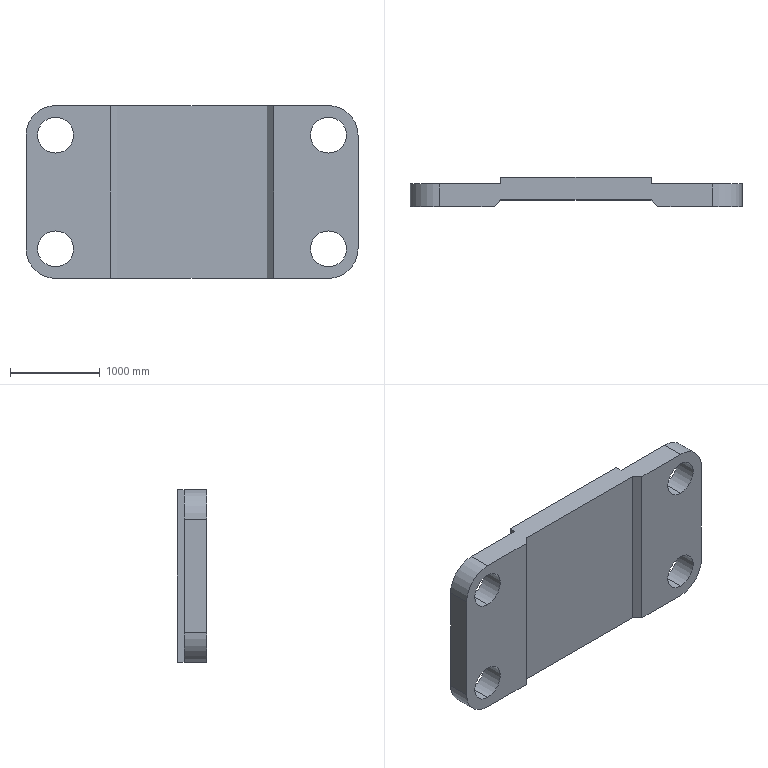Part | SolidWorks | features ICE 3, Extrusion 1 | 1 solid | 26 faces | box 3708 x 330.2 x 1930 mm | volume 1654730858 mm3 | plane 14 | cylinder 12 | commonest cylinder face diameters 401.441 x8 660.4 x4
STEP:
#1=CARTESIAN_POINT('',(-60.,13.,17.098));
#2=VERTEX_POINT('',#1);
#3=CARTESIAN_POINT('',(-60.,13.,32.902));
#4=VERTEX_POINT('',#3);
#5=CARTESIAN_POINT('',(-60.,13.,25.));
#6=DIRECTION('',(0.,1.,0.));
#7=DIRECTION('',(0.,0.,1.));
#8=AXIS2_PLACEMENT_3D('',#5,#6,#7);
#9=CIRCLE('',#8,7.902);
#10=EDGE_CURVE('',#2,#4,#9,.T.);
#11=ORIENTED_EDGE('',*,*,#10,.T.);
#12=CARTESIAN_POINT('',(-60.,3.,32.902));
#13=VERTEX_POINT('',#12);
#14=CARTESIAN_POINT('',(-60.,13.,32.902));
#15=DIRECTION('',(0.,-1.,0.));
#16=VECTOR('',#15,39.37);
#17=LINE('',#14,#16);
#18=EDGE_CURVE('',#4,#13,#17,.T.);
#19=ORIENTED_EDGE('',*,*,#18,.T.);
#20=CARTESIAN_POINT('',(-60.,3.,17.098));
#21=VERTEX_POINT('',#20);
#22=CARTESIAN_POINT('',(-60.,3.,25.));
#23=DIRECTION('',(0.,-1.,0.));
#24=DIRECTION('',(0.,0.,-1.));
#25=AXIS2_PLACEMENT_3D('',#22,#23,#24);
#26=CIRCLE('',#25,7.902);
#27=EDGE_CURVE('',#13,#21,#26,.T.);
#28=ORIENTED_EDGE('',*,*,#27,.T.);
#29=CARTESIAN_POINT('',(-60.,13.,17.098));
#30=DIRECTION('',(0.,-1.,0.));
#31=VECTOR('',#30,39.37);
#32=LINE('',#29,#31);
#33=EDGE_CURVE('',#2,#21,#32,.T.);
#34=ORIENTED_EDGE('',*,*,#33,.F.);
#35=EDGE_LOOP('',(#11,#19,#28,#34));
#36=FACE_OUTER_BOUND('',#35,.T.);
#37=CARTESIAN_POINT('',(-60.,13.,25.));
#38=DIRECTION('',(0.,-1.,0.));
#39=DIRECTION('',(0.,0.,-1.));
#40=AXIS2_PLACEMENT_3D('',#37,#38,#39);
#41=CYLINDRICAL_SURFACE('',#40,7.902);
#42=ADVANCED_FACE('',(#36),#41,.F.);
#43=CARTESIAN_POINT('',(60.,13.,17.098));
#44=VERTEX_POINT('',#43);
#45=CARTESIAN_POINT('',(60.,13.,32.902));
#46=VERTEX_POINT('',#45);
#47=CARTESIAN_POINT('',(60.,13.,25.));
#48=DIRECTION('',(0.,1.,0.));
#49=DIRECTION('',(0.,0.,1.));
#50=AXIS2_PLACEMENT_3D('',#47,#48,#49);
#51=CIRCLE('',#50,7.902);
#52=EDGE_CURVE('',#44,#46,#51,.T.);
#53=ORIENTED_EDGE('',*,*,#52,.T.);
#54=CARTESIAN_POINT('',(60.,3.,32.902));
#55=VERTEX_POINT('',#54);
#56=CARTESIAN_POINT('',(60.,13.,32.902));
#57=DIRECTION('',(0.,-1.,0.));
#58=VECTOR('',#57,39.37);
#59=LINE('',#56,#58);
#60=EDGE_CURVE('',#46,#55,#59,.T.);
#61=ORIENTED_EDGE('',*,*,#60,.T.);
#62=CARTESIAN_POINT('',(60.,3.,17.098));
#63=VERTEX_POINT('',#62);
#64=CARTESIAN_POINT('',(60.,3.,25.));
#65=DIRECTION('',(0.,-1.,0.));
#66=DIRECTION('',(0.,0.,-1.));
#67=AXIS2_PLACEMENT_3D('',#64,#65,#66);
#68=CIRCLE('',#67,7.902);
#69=EDGE_CURVE('',#55,#63,#68,.T.);
#70=ORIENTED_EDGE('',*,*,#69,.T.);
#71=CARTESIAN_POINT('',(60.,13.,17.098));
#72=DIRECTION('',(0.,-1.,0.));
#73=VECTOR('',#72,39.37);
#74=LINE('',#71,#73);
#75=EDGE_CURVE('',#44,#63,#74,.T.);
#76=ORIENTED_EDGE('',*,*,#75,.F.);
#77=EDGE_LOOP('',(#53,#61,#70,#76));
#78=FACE_OUTER_BOUND('',#77,.T.);
#79=CARTESIAN_POINT('',(60.,13.,25.));
#80=DIRECTION('',(0.,-1.,0.));
#81=DIRECTION('',(0.,0.,-1.));
#82=AXIS2_PLACEMENT_3D('',#79,#80,#81);
#83=CYLINDRICAL_SURFACE('',#82,7.902);
#84=ADVANCED_FACE('',(#78),#83,.F.);
#85=CARTESIAN_POINT('',(-60.,13.,-32.902));
#86=VERTEX_POINT('',#85);
#87=CARTESIAN_POINT('',(-60.,13.,-17.098));
#88=VERTEX_POINT('',#87);
#89=CARTESIAN_POINT('',(-60.,13.,-25.));
#90=DIRECTION('',(0.,1.,0.));
#91=DIRECTION('',(0.,0.,1.));
#92=AXIS2_PLACEMENT_3D('',#89,#90,#91);
#93=CIRCLE('',#92,7.902);
#94=EDGE_CURVE('',#86,#88,#93,.T.);
#95=ORIENTED_EDGE('',*,*,#94,.T.);
#96=CARTESIAN_POINT('',(-60.,3.,-17.098));
#97=VERTEX_POINT('',#96);
#98=CARTESIAN_POINT('',(-60.,13.,-17.098));
#99=DIRECTION('',(0.,-1.,0.));
#100=VECTOR('',#99,39.37);
#101=LINE('',#98,#100);
#102=EDGE_CURVE('',#88,#97,#101,.T.);
#103=ORIENTED_EDGE('',*,*,#102,.T.);
#104=CARTESIAN_POINT('',(-60.,3.,-32.902));
#105=VERTEX_POINT('',#104);
#106=CARTESIAN_POINT('',(-60.,3.,-25.));
#107=DIRECTION('',(0.,-1.,0.));
#108=DIRECTION('',(0.,0.,-1.));
#109=AXIS2_PLACEMENT_3D('',#106,#107,#108);
#110=CIRCLE('',#109,7.902);
#111=EDGE_CURVE('',#97,#105,#110,.T.);
#112=ORIENTED_EDGE('',*,*,#111,.T.);
#113=CARTESIAN_POINT('',(-60.,13.,-32.902));
#114=DIRECTION('',(0.,-1.,0.));
#115=VECTOR('',#114,39.37);
#116=LINE('',#113,#115);
#117=EDGE_CURVE('',#86,#105,#116,.T.);
#118=ORIENTED_EDGE('',*,*,#117,.F.);
#119=EDGE_LOOP('',(#95,#103,#112,#118));
#120=FACE_OUTER_BOUND('',#119,.T.);
#121=CARTESIAN_POINT('',(-60.,13.,-25.));
#122=DIRECTION('',(0.,-1.,0.));
#123=DIRECTION('',(0.,0.,-1.));
#124=AXIS2_PLACEMENT_3D('',#121,#122,#123);
#125=CYLINDRICAL_SURFACE('',#124,7.902);
#126=ADVANCED_FACE('',(#120),#125,.F.);
#127=CARTESIAN_POINT('',(60.,13.,-32.902));
#128=VERTEX_POINT('',#127);
#129=CARTESIAN_POINT('',(60.,13.,-17.098));
#130=VERTEX_POINT('',#129);
#131=CARTESIAN_POINT('',(60.,13.,-25.));
#132=DIRECTION('',(0.,1.,0.));
#133=DIRECTION('',(0.,0.,1.));
#134=AXIS2_PLACEMENT_3D('',#131,#132,#133);
#135=CIRCLE('',#134,7.902);
#136=EDGE_CURVE('',#128,#130,#135,.T.);
#137=ORIENTED_EDGE('',*,*,#136,.T.);
#138=CARTESIAN_POINT('',(60.,3.,-17.098));
#139=VERTEX_POINT('',#138);
#140=CARTESIAN_POINT('',(60.,13.,-17.098));
#141=DIRECTION('',(0.,-1.,0.));
#142=VECTOR('',#141,39.37);
#143=LINE('',#140,#142);
#144=EDGE_CURVE('',#130,#139,#143,.T.);
#145=ORIENTED_EDGE('',*,*,#144,.T.);
#146=CARTESIAN_POINT('',(60.,3.,-32.902));
#147=VERTEX_POINT('',#146);
#148=CARTESIAN_POINT('',(60.,3.,-25.));
#149=DIRECTION('',(0.,-1.,0.));
#150=DIRECTION('',(0.,0.,-1.));
#151=AXIS2_PLACEMENT_3D('',#148,#149,#150);
#152=CIRCLE('',#151,7.902);
#153=EDGE_CURVE('',#139,#147,#152,.T.);
#154=ORIENTED_EDGE('',*,*,#153,.T.);
#155=CARTESIAN_POINT('',(60.,13.,-32.902));
#156=DIRECTION('',(0.,-1.,0.));
#157=VECTOR('',#156,39.37);
#158=LINE('',#155,#157);
#159=EDGE_CURVE('',#128,#147,#158,.T.);
#160=ORIENTED_EDGE('',*,*,#159,.F.);
#161=EDGE_LOOP('',(#137,#145,#154,#160));
#162=FACE_OUTER_BOUND('',#161,.T.);
#163=CARTESIAN_POINT('',(60.,13.,-25.));
#164=DIRECTION('',(0.,-1.,0.));
#165=DIRECTION('',(0.,0.,-1.));
#166=AXIS2_PLACEMENT_3D('',#163,#164,#165);
#167=CYLINDRICAL_SURFACE('',#166,7.902);
#168=ADVANCED_FACE('',(#162),#167,.F.);
#169=CARTESIAN_POINT('',(33.,6.,38.));
#170=VERTEX_POINT('',#169);
#171=CARTESIAN_POINT('',(36.,3.,38.));
#172=VERTEX_POINT('',#171);
#173=CARTESIAN_POINT('',(19.5,19.5,38.));
#174=DIRECTION('',(0.7071,-0.7071,0.));
#175=VECTOR('',#174,39.37);
#176=LINE('',#173,#175);
#177=EDGE_CURVE('',#170,#172,#176,.T.);
#178=ORIENTED_EDGE('',*,*,#177,.T.);
#179=CARTESIAN_POINT('',(60.,3.,38.));
#180=VERTEX_POINT('',#179);
#181=CARTESIAN_POINT('',(60.,3.,38.));
#182=DIRECTION('',(-1.,0.,0.));
#183=VECTOR('',#182,39.37);
#184=LINE('',#181,#183);
#185=EDGE_CURVE('',#180,#172,#184,.T.);
#186=ORIENTED_EDGE('',*,*,#185,.F.);
#187=CARTESIAN_POINT('',(60.,13.,38.));
#188=VERTEX_POINT('',#187);
#189=CARTESIAN_POINT('',(60.,13.,38.));
#190=DIRECTION('',(0.,-1.,0.));
#191=VECTOR('',#190,39.37);
#192=LINE('',#189,#191);
#193=EDGE_CURVE('',#188,#180,#192,.T.);
#194=ORIENTED_EDGE('',*,*,#193,.F.);
#195=CARTESIAN_POINT('',(33.,13.,38.));
#196=VERTEX_POINT('',#195);
#197=CARTESIAN_POINT('',(60.,13.,38.));
#198=DIRECTION('',(1.,0.,0.));
#199=VECTOR('',#198,39.37);
#200=LINE('',#197,#199);
#201=EDGE_CURVE('',#196,#188,#200,.T.);
#202=ORIENTED_EDGE('',*,*,#201,.F.);
#203=CARTESIAN_POINT('',(33.,16.,38.));
#204=VERTEX_POINT('',#203);
#205=CARTESIAN_POINT('',(33.,16.,38.));
#206=DIRECTION('',(0.,-1.,0.));
#207=VECTOR('',#206,39.37);
#208=LINE('',#205,#207);
#209=EDGE_CURVE('',#204,#196,#208,.T.);
#210=ORIENTED_EDGE('',*,*,#209,.F.);
#211=CARTESIAN_POINT('',(-33.,16.,38.));
#212=VERTEX_POINT('',#211);
#213=CARTESIAN_POINT('',(33.,16.,38.));
#214=DIRECTION('',(1.,0.,0.));
#215=VECTOR('',#214,39.37);
#216=LINE('',#213,#215);
#217=EDGE_CURVE('',#212,#204,#216,.T.);
#218=ORIENTED_EDGE('',*,*,#217,.F.);
#219=CARTESIAN_POINT('',(-33.,13.,38.));
#220=VERTEX_POINT('',#219);
#221=CARTESIAN_POINT('',(-33.,16.,38.));
#222=DIRECTION('',(0.,-1.,0.));
#223=VECTOR('',#222,39.37);
#224=LINE('',#221,#223);
#225=EDGE_CURVE('',#212,#220,#224,.T.);
#226=ORIENTED_EDGE('',*,*,#225,.T.);
#227=CARTESIAN_POINT('',(-60.,13.,38.));
#228=VERTEX_POINT('',#227);
#229=CARTESIAN_POINT('',(60.,13.,38.));
#230=DIRECTION('',(1.,0.,0.));
#231=VECTOR('',#230,39.37);
#232=LINE('',#229,#231);
#233=EDGE_CURVE('',#228,#220,#232,.T.);
#234=ORIENTED_EDGE('',*,*,#233,.F.);
#235=CARTESIAN_POINT('',(-60.,3.,38.));
#236=VERTEX_POINT('',#235);
#237=CARTESIAN_POINT('',(-60.,13.,38.));
#238=DIRECTION('',(0.,-1.,0.));
#239=VECTOR('',#238,39.37);
#240=LINE('',#237,#239);
#241=EDGE_CURVE('',#228,#236,#240,.T.);
#242=ORIENTED_EDGE('',*,*,#241,.T.);
#243=CARTESIAN_POINT('',(-36.,3.,38.));
#244=VERTEX_POINT('',#243);
#245=CARTESIAN_POINT('',(60.,3.,38.));
#246=DIRECTION('',(-1.,0.,0.));
#247=VECTOR('',#246,39.37);
#248=LINE('',#245,#247);
#249=EDGE_CURVE('',#244,#236,#248,.T.);
#250=ORIENTED_EDGE('',*,*,#249,.F.);
#251=CARTESIAN_POINT('',(-33.,6.,38.));
#252=VERTEX_POINT('',#251);
#253=CARTESIAN_POINT('',(-19.5,19.5,38.));
#254=DIRECTION('',(0.7071,0.7071,0.));
#255=VECTOR('',#254,39.37);
#256=LINE('',#253,#255);
#257=EDGE_CURVE('',#244,#252,#256,.T.);
#258=ORIENTED_EDGE('',*,*,#257,.T.);
#259=CARTESIAN_POINT('',(0.,6.,38.));
#260=DIRECTION('',(-1.,0.,0.));
#261=VECTOR('',#260,39.37);
#262=LINE('',#259,#261);
#263=EDGE_CURVE('',#170,#252,#262,.T.);
#264=ORIENTED_EDGE('',*,*,#263,.F.);
#265=EDGE_LOOP('',(#178,#186,#194,#202,#210,#218,#226,#234,#242,#250,#258,#264));
#266=FACE_OUTER_BOUND('',#265,.T.);
#267=CARTESIAN_POINT('',(60.,13.,38.));
#268=DIRECTION('',(0.,0.,-1.));
#269=DIRECTION('',(-1.,0.,0.));
#270=AXIS2_PLACEMENT_3D('',#267,#268,#269);
#271=PLANE('',#270);
#272=ADVANCED_FACE('',(#266),#271,.F.);
#273=CARTESIAN_POINT('',(33.,6.,-38.));
#274=VERTEX_POINT('',#273);
#275=CARTESIAN_POINT('',(36.,3.,-38.));
#276=VERTEX_POINT('',#275);
#277=CARTESIAN_POINT('',(19.5,19.5,-38.));
#278=DIRECTION('',(0.7071,-0.7071,0.));
#279=VECTOR('',#278,39.37);
#280=LINE('',#277,#279);
#281=EDGE_CURVE('',#274,#276,#280,.T.);
#282=ORIENTED_EDGE('',*,*,#281,.F.);
#283=CARTESIAN_POINT('',(-33.,6.,-38.));
#284=VERTEX_POINT('',#283);
#285=CARTESIAN_POINT('',(0.,6.,-38.));
#286=DIRECTION('',(-1.,0.,0.));
#287=VECTOR('',#286,39.37);
#288=LINE('',#285,#287);
#289=EDGE_CURVE('',#274,#284,#288,.T.);
#290=ORIENTED_EDGE('',*,*,#289,.T.);
#291=CARTESIAN_POINT('',(-36.,3.,-38.));
#292=VERTEX_POINT('',#291);
#293=CARTESIAN_POINT('',(-19.5,19.5,-38.));
#294=DIRECTION('',(0.7071,0.7071,0.));
#295=VECTOR('',#294,39.37);
#296=LINE('',#293,#295);
#297=EDGE_CURVE('',#292,#284,#296,.T.);
#298=ORIENTED_EDGE('',*,*,#297,.F.);
#299=CARTESIAN_POINT('',(-60.,3.,-38.));
#300=VERTEX_POINT('',#299);
#301=CARTESIAN_POINT('',(-60.,3.,-38.));
#302=DIRECTION('',(1.,0.,0.));
#303=VECTOR('',#302,39.37);
#304=LINE('',#301,#303);
#305=EDGE_CURVE('',#300,#292,#304,.T.);
#306=ORIENTED_EDGE('',*,*,#305,.F.);
#307=CARTESIAN_POINT('',(-60.,13.,-38.));
#308=VERTEX_POINT('',#307);
#309=CARTESIAN_POINT('',(-60.,13.,-38.));
#310=DIRECTION('',(0.,-1.,0.));
#311=VECTOR('',#310,39.37);
#312=LINE('',#309,#311);
#313=EDGE_CURVE('',#308,#300,#312,.T.);
#314=ORIENTED_EDGE('',*,*,#313,.F.);
#315=CARTESIAN_POINT('',(-33.,13.,-38.));
#316=VERTEX_POINT('',#315);
#317=CARTESIAN_POINT('',(60.,13.,-38.));
#318=DIRECTION('',(-1.,0.,0.));
#319=VECTOR('',#318,39.37);
#320=LINE('',#317,#319);
#321=EDGE_CURVE('',#316,#308,#320,.T.);
#322=ORIENTED_EDGE('',*,*,#321,.F.);
#323=CARTESIAN_POINT('',(-33.,16.,-38.));
#324=VERTEX_POINT('',#323);
#325=CARTESIAN_POINT('',(-33.,16.,-38.));
#326=DIRECTION('',(0.,-1.,0.));
#327=VECTOR('',#326,39.37);
#328=LINE('',#325,#327);
#329=EDGE_CURVE('',#324,#316,#328,.T.);
#330=ORIENTED_EDGE('',*,*,#329,.F.);
#331=CARTESIAN_POINT('',(33.,16.,-38.));
#332=VERTEX_POINT('',#331);
#333=CARTESIAN_POINT('',(-33.,16.,-38.));
#334=DIRECTION('',(-1.,0.,0.));
#335=VECTOR('',#334,39.37);
#336=LINE('',#333,#335);
#337=EDGE_CURVE('',#332,#324,#336,.T.);
#338=ORIENTED_EDGE('',*,*,#337,.F.);
#339=CARTESIAN_POINT('',(33.,13.,-38.));
#340=VERTEX_POINT('',#339);
#341=CARTESIAN_POINT('',(33.,16.,-38.));
#342=DIRECTION('',(0.,-1.,0.));
#343=VECTOR('',#342,39.37);
#344=LINE('',#341,#343);
#345=EDGE_CURVE('',#332,#340,#344,.T.);
#346=ORIENTED_EDGE('',*,*,#345,.T.);
#347=CARTESIAN_POINT('',(60.,13.,-38.));
#348=VERTEX_POINT('',#347);
#349=CARTESIAN_POINT('',(60.,13.,-38.));
#350=DIRECTION('',(-1.,0.,0.));
#351=VECTOR('',#350,39.37);
#352=LINE('',#349,#351);
#353=EDGE_CURVE('',#348,#340,#352,.T.);
#354=ORIENTED_EDGE('',*,*,#353,.F.);
#355=CARTESIAN_POINT('',(60.,3.,-38.));
#356=VERTEX_POINT('',#355);
#357=CARTESIAN_POINT('',(60.,13.,-38.));
#358=DIRECTION('',(0.,-1.,0.));
#359=VECTOR('',#358,39.37);
#360=LINE('',#357,#359);
#361=EDGE_CURVE('',#348,#356,#360,.T.);
#362=ORIENTED_EDGE('',*,*,#361,.T.);
#363=CARTESIAN_POINT('',(-60.,3.,-38.));
#364=DIRECTION('',(1.,0.,0.));
#365=VECTOR('',#364,39.37);
#366=LINE('',#363,#365);
#367=EDGE_CURVE('',#276,#356,#366,.T.);
#368=ORIENTED_EDGE('',*,*,#367,.F.);
#369=EDGE_LOOP('',(#282,#290,#298,#306,#314,#322,#330,#338,#346,#354,#362,#368));
#370=FACE_OUTER_BOUND('',#369,.T.);
#371=CARTESIAN_POINT('',(60.,13.,-38.));
#372=DIRECTION('',(0.,0.,1.));
#373=DIRECTION('',(1.,0.,0.));
#374=AXIS2_PLACEMENT_3D('',#371,#372,#373);
#375=PLANE('',#374);
#376=ADVANCED_FACE('',(#370),#375,.F.);
#377=CARTESIAN_POINT('',(60.,3.,-25.));
#378=DIRECTION('',(0.,-1.,0.));
#379=DIRECTION('',(0.,0.,-1.));
#380=AXIS2_PLACEMENT_3D('',#377,#378,#379);
#381=CIRCLE('',#380,7.902);
#382=EDGE_CURVE('',#147,#139,#381,.T.);
#383=ORIENTED_EDGE('',*,*,#382,.F.);
#384=ORIENTED_EDGE('',*,*,#153,.F.);
#385=EDGE_LOOP('',(#383,#384));
#386=FACE_BOUND('',#385,.T.);
#387=CARTESIAN_POINT('',(60.,3.,25.));
#388=DIRECTION('',(0.,-1.,0.));
#389=DIRECTION('',(0.,0.,-1.));
#390=AXIS2_PLACEMENT_3D('',#387,#388,#389);
#391=CIRCLE('',#390,7.902);
#392=EDGE_CURVE('',#63,#55,#391,.T.);
#393=ORIENTED_EDGE('',*,*,#392,.F.);
#394=ORIENTED_EDGE('',*,*,#69,.F.);
#395=EDGE_LOOP('',(#393,#394));
#396=FACE_BOUND('',#395,.T.);
#397=ORIENTED_EDGE('',*,*,#185,.T.);
#398=CARTESIAN_POINT('',(36.,3.,-38.));
#399=DIRECTION('',(0.,0.,1.));
#400=VECTOR('',#399,39.37);
#401=LINE('',#398,#400);
#402=EDGE_CURVE('',#276,#172,#401,.T.);
#403=ORIENTED_EDGE('',*,*,#402,.F.);
#404=ORIENTED_EDGE('',*,*,#367,.T.);
#405=CARTESIAN_POINT('',(73.,3.,-25.));
#406=VERTEX_POINT('',#405);
#407=CARTESIAN_POINT('',(60.,3.,-25.));
#408=DIRECTION('',(0.,-1.,0.));
#409=DIRECTION('',(0.,0.,-1.));
#410=AXIS2_PLACEMENT_3D('',#407,#408,#409);
#411=CIRCLE('',#410,13.);
#412=EDGE_CURVE('',#356,#406,#411,.T.);
#413=ORIENTED_EDGE('',*,*,#412,.T.);
#414=CARTESIAN_POINT('',(73.,3.,25.));
#415=VERTEX_POINT('',#414);
#416=CARTESIAN_POINT('',(73.,3.,-25.));
#417=DIRECTION('',(0.,0.,1.));
#418=VECTOR('',#417,39.37);
#419=LINE('',#416,#418);
#420=EDGE_CURVE('',#406,#415,#419,.T.);
#421=ORIENTED_EDGE('',*,*,#420,.T.);
#422=CARTESIAN_POINT('',(60.,3.,25.));
#423=DIRECTION('',(0.,-1.,0.));
#424=DIRECTION('',(0.,0.,-1.));
#425=AXIS2_PLACEMENT_3D('',#422,#423,#424);
#426=CIRCLE('',#425,13.);
#427=EDGE_CURVE('',#415,#180,#426,.T.);
#428=ORIENTED_EDGE('',*,*,#427,.T.);
#429=EDGE_LOOP('',(#397,#403,#404,#413,#421,#428));
#430=FACE_OUTER_BOUND('',#429,.T.);
#431=CARTESIAN_POINT('',(-60.,3.,-25.));
#432=DIRECTION('',(0.,-1.,0.));
#433=DIRECTION('',(0.,0.,-1.));
#434=AXIS2_PLACEMENT_3D('',#431,#432,#433);
#435=PLANE('',#434);
#436=ADVANCED_FACE('',(#386,#396,#430),#435,.T.);
#437=CARTESIAN_POINT('',(-60.,3.,25.));
#438=DIRECTION('',(0.,-1.,0.));
#439=DIRECTION('',(0.,0.,-1.));
#440=AXIS2_PLACEMENT_3D('',#437,#438,#439);
#441=CIRCLE('',#440,7.902);
#442=EDGE_CURVE('',#21,#13,#441,.T.);
#443=ORIENTED_EDGE('',*,*,#442,.F.);
#444=ORIENTED_EDGE('',*,*,#27,.F.);
#445=EDGE_LOOP('',(#443,#444));
#446=FACE_BOUND('',#445,.T.);
#447=CARTESIAN_POINT('',(-60.,3.,-25.));
#448=DIRECTION('',(0.,-1.,0.));
#449=DIRECTION('',(0.,0.,-1.));
#450=AXIS2_PLACEMENT_3D('',#447,#448,#449);
#451=CIRCLE('',#450,7.902);
#452=EDGE_CURVE('',#105,#97,#451,.T.);
#453=ORIENTED_EDGE('',*,*,#452,.F.);
#454=ORIENTED_EDGE('',*,*,#111,.F.);
#455=EDGE_LOOP('',(#453,#454));
#456=FACE_BOUND('',#455,.T.);
#457=ORIENTED_EDGE('',*,*,#305,.T.);
#458=CARTESIAN_POINT('',(-36.,3.,-38.));
#459=DIRECTION('',(0.,0.,1.));
#460=VECTOR('',#459,39.37);
#461=LINE('',#458,#460);
#462=EDGE_CURVE('',#292,#244,#461,.T.);
#463=ORIENTED_EDGE('',*,*,#462,.T.);
#464=ORIENTED_EDGE('',*,*,#249,.T.);
#465=CARTESIAN_POINT('',(-73.,3.,25.));
#466=VERTEX_POINT('',#465);
#467=CARTESIAN_POINT('',(-60.,3.,25.));
#468=DIRECTION('',(0.,-1.,0.));
#469=DIRECTION('',(0.,0.,-1.));
#470=AXIS2_PLACEMENT_3D('',#467,#468,#469);
#471=CIRCLE('',#470,13.);
#472=EDGE_CURVE('',#236,#466,#471,.T.);
#473=ORIENTED_EDGE('',*,*,#472,.T.);
#474=CARTESIAN_POINT('',(-73.,3.,-25.));
#475=VERTEX_POINT('',#474);
#476=CARTESIAN_POINT('',(-73.,3.,25.));
#477=DIRECTION('',(0.,0.,-1.));
#478=VECTOR('',#477,39.37);
#479=LINE('',#476,#478);
#480=EDGE_CURVE('',#466,#475,#479,.T.);
#481=ORIENTED_EDGE('',*,*,#480,.T.);
#482=CARTESIAN_POINT('',(-60.,3.,-25.));
#483=DIRECTION('',(0.,-1.,0.));
#484=DIRECTION('',(0.,0.,-1.));
#485=AXIS2_PLACEMENT_3D('',#482,#483,#484);
#486=CIRCLE('',#485,13.);
#487=EDGE_CURVE('',#475,#300,#486,.T.);
#488=ORIENTED_EDGE('',*,*,#487,.T.);
#489=EDGE_LOOP('',(#457,#463,#464,#473,#481,#488));
#490=FACE_OUTER_BOUND('',#489,.T.);
#491=CARTESIAN_POINT('',(-60.,3.,-25.));
#492=DIRECTION('',(0.,-1.,0.));
#493=DIRECTION('',(0.,0.,-1.));
#494=AXIS2_PLACEMENT_3D('',#491,#492,#493);
#495=PLANE('',#494);
#496=ADVANCED_FACE('',(#446,#456,#490),#495,.T.);
#497=ORIENTED_EDGE('',*,*,#487,.F.);
#498=CARTESIAN_POINT('',(-73.,13.,-25.));
#499=VERTEX_POINT('',#498);
#500=CARTESIAN_POINT('',(-73.,13.,-25.));
#501=DIRECTION('',(0.,-1.,0.));
#502=VECTOR('',#501,39.37);
#503=LINE('',#500,#502);
#504=EDGE_CURVE('',#499,#475,#503,.T.);
#505=ORIENTED_EDGE('',*,*,#504,.F.);
#506=CARTESIAN_POINT('',(-60.,13.,-25.));
#507=DIRECTION('',(0.,1.,0.));
#508=DIRECTION('',(0.,0.,1.));
#509=AXIS2_PLACEMENT_3D('',#506,#507,#508);
#510=CIRCLE('',#509,13.);
#511=EDGE_CURVE('',#308,#499,#510,.T.);
#512=ORIENTED_EDGE('',*,*,#511,.F.);
#513=ORIENTED_EDGE('',*,*,#313,.T.);
#514=EDGE_LOOP('',(#497,#505,#512,#513));
#515=FACE_OUTER_BOUND('',#514,.T.);
#516=CARTESIAN_POINT('',(-60.,13.,-25.));
#517=DIRECTION('',(0.,-1.,0.));
#518=DIRECTION('',(0.,0.,-1.));
#519=AXIS2_PLACEMENT_3D('',#516,#517,#518);
#520=CYLINDRICAL_SURFACE('',#519,13.);
#521=ADVANCED_FACE('',(#515),#520,.T.);
#522=ORIENTED_EDGE('',*,*,#480,.F.);
#523=CARTESIAN_POINT('',(-73.,13.,25.));
#524=VERTEX_POINT('',#523);
#525=CARTESIAN_POINT('',(-73.,13.,25.));
#526=DIRECTION('',(0.,-1.,0.));
#527=VECTOR('',#526,39.37);
#528=LINE('',#525,#527);
#529=EDGE_CURVE('',#524,#466,#528,.T.);
#530=ORIENTED_EDGE('',*,*,#529,.F.);
#531=CARTESIAN_POINT('',(-73.,13.,-25.));
#532=DIRECTION('',(0.,0.,1.));
#533=VECTOR('',#532,39.37);
#534=LINE('',#531,#533);
#535=EDGE_CURVE('',#499,#524,#534,.T.);
#536=ORIENTED_EDGE('',*,*,#535,.F.);
#537=ORIENTED_EDGE('',*,*,#504,.T.);
#538=EDGE_LOOP('',(#522,#530,#536,#537));
#539=FACE_OUTER_BOUND('',#538,.T.);
#540=CARTESIAN_POINT('',(-73.,13.,-25.));
#541=DIRECTION('',(1.,0.,0.));
#542=DIRECTION('',(0.,0.,-1.));
#543=AXIS2_PLACEMENT_3D('',#540,#541,#542);
#544=PLANE('',#543);
#545=ADVANCED_FACE('',(#539),#544,.F.);
#546=ORIENTED_EDGE('',*,*,#472,.F.);
#547=ORIENTED_EDGE('',*,*,#241,.F.);
#548=CARTESIAN_POINT('',(-60.,13.,25.));
#549=DIRECTION('',(0.,1.,0.));
#550=DIRECTION('',(0.,0.,-1.));
#551=AXIS2_PLACEMENT_3D('',#548,#549,#550);
#552=CIRCLE('',#551,13.);
#553=EDGE_CURVE('',#524,#228,#552,.T.);
#554=ORIENTED_EDGE('',*,*,#553,.F.);
#555=ORIENTED_EDGE('',*,*,#529,.T.);
#556=EDGE_LOOP('',(#546,#547,#554,#555));
#557=FACE_OUTER_BOUND('',#556,.T.);
#558=CARTESIAN_POINT('',(-60.,13.,25.));
#559=DIRECTION('',(0.,-1.,0.));
#560=DIRECTION('',(0.,0.,-1.));
#561=AXIS2_PLACEMENT_3D('',#558,#559,#560);
#562=CYLINDRICAL_SURFACE('',#561,13.);
#563=ADVANCED_FACE('',(#557),#562,.T.);
#564=ORIENTED_EDGE('',*,*,#427,.F.);
#565=CARTESIAN_POINT('',(73.,13.,25.));
#566=VERTEX_POINT('',#565);
#567=CARTESIAN_POINT('',(73.,13.,25.));
#568=DIRECTION('',(0.,-1.,0.));
#569=VECTOR('',#568,39.37);
#570=LINE('',#567,#569);
#571=EDGE_CURVE('',#566,#415,#570,.T.);
#572=ORIENTED_EDGE('',*,*,#571,.F.);
#573=CARTESIAN_POINT('',(60.,13.,25.));
#574=DIRECTION('',(0.,1.,0.));
#575=DIRECTION('',(0.,0.,-1.));
#576=AXIS2_PLACEMENT_3D('',#573,#574,#575);
#577=CIRCLE('',#576,13.);
#578=EDGE_CURVE('',#188,#566,#577,.T.);
#579=ORIENTED_EDGE('',*,*,#578,.F.);
#580=ORIENTED_EDGE('',*,*,#193,.T.);
#581=EDGE_LOOP('',(#564,#572,#579,#580));
#582=FACE_OUTER_BOUND('',#581,.T.);
#583=CARTESIAN_POINT('',(60.,13.,25.));
#584=DIRECTION('',(0.,-1.,0.));
#585=DIRECTION('',(0.,0.,-1.));
#586=AXIS2_PLACEMENT_3D('',#583,#584,#585);
#587=CYLINDRICAL_SURFACE('',#586,13.);
#588=ADVANCED_FACE('',(#582),#587,.T.);
#589=ORIENTED_EDGE('',*,*,#420,.F.);
#590=CARTESIAN_POINT('',(73.,13.,-25.));
#591=VERTEX_POINT('',#590);
#592=CARTESIAN_POINT('',(73.,13.,-25.));
#593=DIRECTION('',(0.,-1.,0.));
#594=VECTOR('',#593,39.37);
#595=LINE('',#592,#594);
#596=EDGE_CURVE('',#591,#406,#595,.T.);
#597=ORIENTED_EDGE('',*,*,#596,.F.);
#598=CARTESIAN_POINT('',(73.,13.,-25.));
#599=DIRECTION('',(0.,0.,-1.));
#600=VECTOR('',#599,39.37);
#601=LINE('',#598,#600);
#602=EDGE_CURVE('',#566,#591,#601,.T.);
#603=ORIENTED_EDGE('',*,*,#602,.F.);
#604=ORIENTED_EDGE('',*,*,#571,.T.);
#605=EDGE_LOOP('',(#589,#597,#603,#604));
#606=FACE_OUTER_BOUND('',#605,.T.);
#607=CARTESIAN_POINT('',(73.,13.,-25.));
#608=DIRECTION('',(-1.,0.,0.));
#609=DIRECTION('',(0.,0.,1.));
#610=AXIS2_PLACEMENT_3D('',#607,#608,#609);
#611=PLANE('',#610);
#612=ADVANCED_FACE('',(#606),#611,.F.);
#613=ORIENTED_EDGE('',*,*,#412,.F.);
#614=ORIENTED_EDGE('',*,*,#361,.F.);
#615=CARTESIAN_POINT('',(60.,13.,-25.));
#616=DIRECTION('',(0.,1.,0.));
#617=DIRECTION('',(0.,0.,-1.));
#618=AXIS2_PLACEMENT_3D('',#615,#616,#617);
#619=CIRCLE('',#618,13.);
#620=EDGE_CURVE('',#591,#348,#619,.T.);
#621=ORIENTED_EDGE('',*,*,#620,.F.);
#622=ORIENTED_EDGE('',*,*,#596,.T.);
#623=EDGE_LOOP('',(#613,#614,#621,#622));
#624=FACE_OUTER_BOUND('',#623,.T.);
#625=CARTESIAN_POINT('',(60.,13.,-25.));
#626=DIRECTION('',(0.,-1.,0.));
#627=DIRECTION('',(0.,0.,-1.));
#628=AXIS2_PLACEMENT_3D('',#625,#626,#627);
#629=CYLINDRICAL_SURFACE('',#628,13.);
#630=ADVANCED_FACE('',(#624),#629,.T.);
#631=ORIENTED_EDGE('',*,*,#144,.F.);
#632=CARTESIAN_POINT('',(60.,13.,-25.));
#633=DIRECTION('',(0.,1.,0.));
#634=DIRECTION('',(0.,0.,1.));
#635=AXIS2_PLACEMENT_3D('',#632,#633,#634);
#636=CIRCLE('',#635,7.902);
#637=EDGE_CURVE('',#130,#128,#636,.T.);
#638=ORIENTED_EDGE('',*,*,#637,.T.);
#639=ORIENTED_EDGE('',*,*,#159,.T.);
#640=ORIENTED_EDGE('',*,*,#382,.T.);
#641=EDGE_LOOP('',(#631,#638,#639,#640));
#642=FACE_OUTER_BOUND('',#641,.T.);
#643=CARTESIAN_POINT('',(60.,13.,-25.));
#644=DIRECTION('',(0.,-1.,0.));
#645=DIRECTION('',(0.,0.,-1.));
#646=AXIS2_PLACEMENT_3D('',#643,#644,#645);
#647=CYLINDRICAL_SURFACE('',#646,7.902);
#648=ADVANCED_FACE('',(#642),#647,.F.);
#649=ORIENTED_EDGE('',*,*,#102,.F.);
#650=CARTESIAN_POINT('',(-60.,13.,-25.));
#651=DIRECTION('',(0.,1.,0.));
#652=DIRECTION('',(0.,0.,1.));
#653=AXIS2_PLACEMENT_3D('',#650,#651,#652);
#654=CIRCLE('',#653,7.902);
#655=EDGE_CURVE('',#88,#86,#654,.T.);
#656=ORIENTED_EDGE('',*,*,#655,.T.);
#657=ORIENTED_EDGE('',*,*,#117,.T.);
#658=ORIENTED_EDGE('',*,*,#452,.T.);
#659=EDGE_LOOP('',(#649,#656,#657,#658));
#660=FACE_OUTER_BOUND('',#659,.T.);
#661=CARTESIAN_POINT('',(-60.,13.,-25.));
#662=DIRECTION('',(0.,-1.,0.));
#663=DIRECTION('',(0.,0.,-1.));
#664=AXIS2_PLACEMENT_3D('',#661,#662,#663);
#665=CYLINDRICAL_SURFACE('',#664,7.902);
#666=ADVANCED_FACE('',(#660),#665,.F.);
#667=ORIENTED_EDGE('',*,*,#60,.F.);
#668=CARTESIAN_POINT('',(60.,13.,25.));
#669=DIRECTION('',(0.,1.,0.));
#670=DIRECTION('',(0.,0.,1.));
#671=AXIS2_PLACEMENT_3D('',#668,#669,#670);
#672=CIRCLE('',#671,7.902);
#673=EDGE_CURVE('',#46,#44,#672,.T.);
#674=ORIENTED_EDGE('',*,*,#673,.T.);
#675=ORIENTED_EDGE('',*,*,#75,.T.);
#676=ORIENTED_EDGE('',*,*,#392,.T.);
#677=EDGE_LOOP('',(#667,#674,#675,#676));
#678=FACE_OUTER_BOUND('',#677,.T.);
#679=CARTESIAN_POINT('',(60.,13.,25.));
#680=DIRECTION('',(0.,-1.,0.));
#681=DIRECTION('',(0.,0.,-1.));
#682=AXIS2_PLACEMENT_3D('',#679,#680,#681);
#683=CYLINDRICAL_SURFACE('',#682,7.902);
#684=ADVANCED_FACE('',(#678),#683,.F.);
#685=ORIENTED_EDGE('',*,*,#18,.F.);
#686=CARTESIAN_POINT('',(-60.,13.,25.));
#687=DIRECTION('',(0.,1.,0.));
#688=DIRECTION('',(0.,0.,1.));
#689=AXIS2_PLACEMENT_3D('',#686,#687,#688);
#690=CIRCLE('',#689,7.902);
#691=EDGE_CURVE('',#4,#2,#690,.T.);
#692=ORIENTED_EDGE('',*,*,#691,.T.);
#693=ORIENTED_EDGE('',*,*,#33,.T.);
#694=ORIENTED_EDGE('',*,*,#442,.T.);
#695=EDGE_LOOP('',(#685,#692,#693,#694));
#696=FACE_OUTER_BOUND('',#695,.T.);
#697=CARTESIAN_POINT('',(-60.,13.,25.));
#698=DIRECTION('',(0.,-1.,0.));
#699=DIRECTION('',(0.,0.,-1.));
#700=AXIS2_PLACEMENT_3D('',#697,#698,#699);
#701=CYLINDRICAL_SURFACE('',#700,7.902);
#702=ADVANCED_FACE('',(#696),#701,.F.);
#703=CARTESIAN_POINT('',(33.,13.,-38.));
#704=DIRECTION('',(0.,0.,-1.));
#705=VECTOR('',#704,39.37);
#706=LINE('',#703,#705);
#707=EDGE_CURVE('',#196,#340,#706,.T.);
#708=ORIENTED_EDGE('',*,*,#707,.F.);
#709=ORIENTED_EDGE('',*,*,#201,.T.);
#710=ORIENTED_EDGE('',*,*,#578,.T.);
#711=ORIENTED_EDGE('',*,*,#602,.T.);
#712=ORIENTED_EDGE('',*,*,#620,.T.);
#713=ORIENTED_EDGE('',*,*,#353,.T.);
#714=EDGE_LOOP('',(#708,#709,#710,#711,#712,#713));
#715=FACE_OUTER_BOUND('',#714,.T.);
#716=ORIENTED_EDGE('',*,*,#136,.F.);
#717=ORIENTED_EDGE('',*,*,#637,.F.);
#718=EDGE_LOOP('',(#716,#717));
#719=FACE_BOUND('',#718,.T.);
#720=ORIENTED_EDGE('',*,*,#52,.F.);
#721=ORIENTED_EDGE('',*,*,#673,.F.);
#722=EDGE_LOOP('',(#720,#721));
#723=FACE_BOUND('',#722,.T.);
#724=CARTESIAN_POINT('',(-60.,13.,-25.));
#725=DIRECTION('',(0.,1.,0.));
#726=DIRECTION('',(0.,0.,1.));
#727=AXIS2_PLACEMENT_3D('',#724,#725,#726);
#728=PLANE('',#727);
#729=ADVANCED_FACE('',(#715,#719,#723),#728,.T.);
#730=CARTESIAN_POINT('',(-33.,13.,-38.));
#731=DIRECTION('',(0.,0.,1.));
#732=VECTOR('',#731,39.37);
#733=LINE('',#730,#732);
#734=EDGE_CURVE('',#316,#220,#733,.T.);
#735=ORIENTED_EDGE('',*,*,#734,.F.);
#736=ORIENTED_EDGE('',*,*,#321,.T.);
#737=ORIENTED_EDGE('',*,*,#511,.T.);
#738=ORIENTED_EDGE('',*,*,#535,.T.);
#739=ORIENTED_EDGE('',*,*,#553,.T.);
#740=ORIENTED_EDGE('',*,*,#233,.T.);
#741=EDGE_LOOP('',(#735,#736,#737,#738,#739,#740));
#742=FACE_OUTER_BOUND('',#741,.T.);
#743=ORIENTED_EDGE('',*,*,#94,.F.);
#744=ORIENTED_EDGE('',*,*,#655,.F.);
#745=EDGE_LOOP('',(#743,#744));
#746=FACE_BOUND('',#745,.T.);
#747=ORIENTED_EDGE('',*,*,#10,.F.);
#748=ORIENTED_EDGE('',*,*,#691,.F.);
#749=EDGE_LOOP('',(#747,#748));
#750=FACE_BOUND('',#749,.T.);
#751=CARTESIAN_POINT('',(-60.,13.,-25.));
#752=DIRECTION('',(0.,1.,0.));
#753=DIRECTION('',(0.,0.,1.));
#754=AXIS2_PLACEMENT_3D('',#751,#752,#753);
#755=PLANE('',#754);
#756=ADVANCED_FACE('',(#742,#746,#750),#755,.T.);
#757=ORIENTED_EDGE('',*,*,#734,.T.);
#758=ORIENTED_EDGE('',*,*,#225,.F.);
#759=CARTESIAN_POINT('',(-33.,16.,-38.));
#760=DIRECTION('',(0.,0.,1.));
#761=VECTOR('',#760,39.37);
#762=LINE('',#759,#761);
#763=EDGE_CURVE('',#324,#212,#762,.T.);
#764=ORIENTED_EDGE('',*,*,#763,.F.);
#765=ORIENTED_EDGE('',*,*,#329,.T.);
#766=EDGE_LOOP('',(#757,#758,#764,#765));
#767=FACE_OUTER_BOUND('',#766,.T.);
#768=CARTESIAN_POINT('',(-33.,16.,-38.));
#769=DIRECTION('',(1.,0.,0.));
#770=DIRECTION('',(0.,0.,-1.));
#771=AXIS2_PLACEMENT_3D('',#768,#769,#770);
#772=PLANE('',#771);
#773=ADVANCED_FACE('',(#767),#772,.F.);
#774=ORIENTED_EDGE('',*,*,#707,.T.);
#775=ORIENTED_EDGE('',*,*,#345,.F.);
#776=CARTESIAN_POINT('',(33.,16.,-38.));
#777=DIRECTION('',(0.,0.,-1.));
#778=VECTOR('',#777,39.37);
#779=LINE('',#776,#778);
#780=EDGE_CURVE('',#204,#332,#779,.T.);
#781=ORIENTED_EDGE('',*,*,#780,.F.);
#782=ORIENTED_EDGE('',*,*,#209,.T.);
#783=EDGE_LOOP('',(#774,#775,#781,#782));
#784=FACE_OUTER_BOUND('',#783,.T.);
#785=CARTESIAN_POINT('',(33.,16.,-38.));
#786=DIRECTION('',(-1.,0.,0.));
#787=DIRECTION('',(0.,0.,1.));
#788=AXIS2_PLACEMENT_3D('',#785,#786,#787);
#789=PLANE('',#788);
#790=ADVANCED_FACE('',(#784),#789,.F.);
#791=ORIENTED_EDGE('',*,*,#337,.T.);
#792=ORIENTED_EDGE('',*,*,#763,.T.);
#793=ORIENTED_EDGE('',*,*,#217,.T.);
#794=ORIENTED_EDGE('',*,*,#780,.T.);
#795=EDGE_LOOP('',(#791,#792,#793,#794));
#796=FACE_OUTER_BOUND('',#795,.T.);
#797=CARTESIAN_POINT('',(0.,16.,0.));
#798=DIRECTION('',(0.,-1.,0.));
#799=DIRECTION('',(0.,0.,-1.));
#800=AXIS2_PLACEMENT_3D('',#797,#798,#799);
#801=PLANE('',#800);
#802=ADVANCED_FACE('',(#796),#801,.F.);
#803=ORIENTED_EDGE('',*,*,#177,.F.);
#804=CARTESIAN_POINT('',(33.,6.,-38.));
#805=DIRECTION('',(0.,0.,1.));
#806=VECTOR('',#805,39.37);
#807=LINE('',#804,#806);
#808=EDGE_CURVE('',#274,#170,#807,.T.);
#809=ORIENTED_EDGE('',*,*,#808,.F.);
#810=ORIENTED_EDGE('',*,*,#281,.T.);
#811=ORIENTED_EDGE('',*,*,#402,.T.);
#812=EDGE_LOOP('',(#803,#809,#810,#811));
#813=FACE_OUTER_BOUND('',#812,.T.);
#814=CARTESIAN_POINT('',(19.5,19.5,-38.));
#815=DIRECTION('',(-0.7071,-0.7071,0.));
#816=DIRECTION('',(0.7071,-0.7071,0.));
#817=AXIS2_PLACEMENT_3D('',#814,#815,#816);
#818=PLANE('',#817);
#819=ADVANCED_FACE('',(#813),#818,.T.);
#820=ORIENTED_EDGE('',*,*,#257,.F.);
#821=ORIENTED_EDGE('',*,*,#462,.F.);
#822=ORIENTED_EDGE('',*,*,#297,.T.);
#823=CARTESIAN_POINT('',(-33.,6.,-38.));
#824=DIRECTION('',(0.,0.,1.));
#825=VECTOR('',#824,39.37);
#826=LINE('',#823,#825);
#827=EDGE_CURVE('',#284,#252,#826,.T.);
#828=ORIENTED_EDGE('',*,*,#827,.T.);
#829=EDGE_LOOP('',(#820,#821,#822,#828));
#830=FACE_OUTER_BOUND('',#829,.T.);
#831=CARTESIAN_POINT('',(-19.5,19.5,-38.));
#832=DIRECTION('',(0.7071,-0.7071,0.));
#833=DIRECTION('',(0.7071,0.7071,0.));
#834=AXIS2_PLACEMENT_3D('',#831,#832,#833);
#835=PLANE('',#834);
#836=ADVANCED_FACE('',(#830),#835,.T.);
#837=ORIENTED_EDGE('',*,*,#263,.T.);
#838=ORIENTED_EDGE('',*,*,#827,.F.);
#839=ORIENTED_EDGE('',*,*,#289,.F.);
#840=ORIENTED_EDGE('',*,*,#808,.T.);
#841=EDGE_LOOP('',(#837,#838,#839,#840));
#842=FACE_OUTER_BOUND('',#841,.T.);
#843=CARTESIAN_POINT('',(0.,6.,-38.));
#844=DIRECTION('',(0.,1.,0.));
#845=DIRECTION('',(0.,0.,1.));
#846=AXIS2_PLACEMENT_3D('',#843,#844,#845);
#847=PLANE('',#846);
#848=ADVANCED_FACE('',(#842),#847,.F.);
#849=CLOSED_SHELL('',(#42,#84,#126,#168,#272,#376,#436,#496,#521,#545,#563,#588,#612,#630,#648,#666,#684,#702,#729,#756,#773,#790,#802,#819,#836,#848));
#850=MANIFOLD_SOLID_BREP('',#849);
#851=CARTESIAN_POINT('',(0.,0.,0.));
#852=DIRECTION('',(0.,0.,1.));
#853=DIRECTION('',(1.,0.,0.));
#854=AXIS2_PLACEMENT_3D('',#851,#852,#853);
#855=(LENGTH_UNIT()NAMED_UNIT(*)SI_UNIT($,.METRE.));
#856=LENGTH_MEASURE_WITH_UNIT(LENGTH_MEASURE(0.0254),#855);
#857=DIMENSIONAL_EXPONENTS(1.,0.,0.,0.,0.,0.,0.);
#858=(CONVERSION_BASED_UNIT('INCH',#856)LENGTH_UNIT()NAMED_UNIT(#857));
#859=UNCERTAINTY_MEASURE_WITH_UNIT(LENGTH_MEASURE(0.00001),#858,'','');
#860=(NAMED_UNIT(*)PLANE_ANGLE_UNIT()SI_UNIT($,.RADIAN.));
#861=(NAMED_UNIT(*)SI_UNIT($,.STERADIAN.)SOLID_ANGLE_UNIT());
#862=(GEOMETRIC_REPRESENTATION_CONTEXT(3)GLOBAL_UNCERTAINTY_ASSIGNED_CONTEXT((#859))GLOBAL_UNIT_ASSIGNED_CONTEXT((#858,#860,#861))REPRESENTATION_CONTEXT('',''));
#863=ADVANCED_BREP_SHAPE_REPRESENTATION('',(#850,#854),#862);